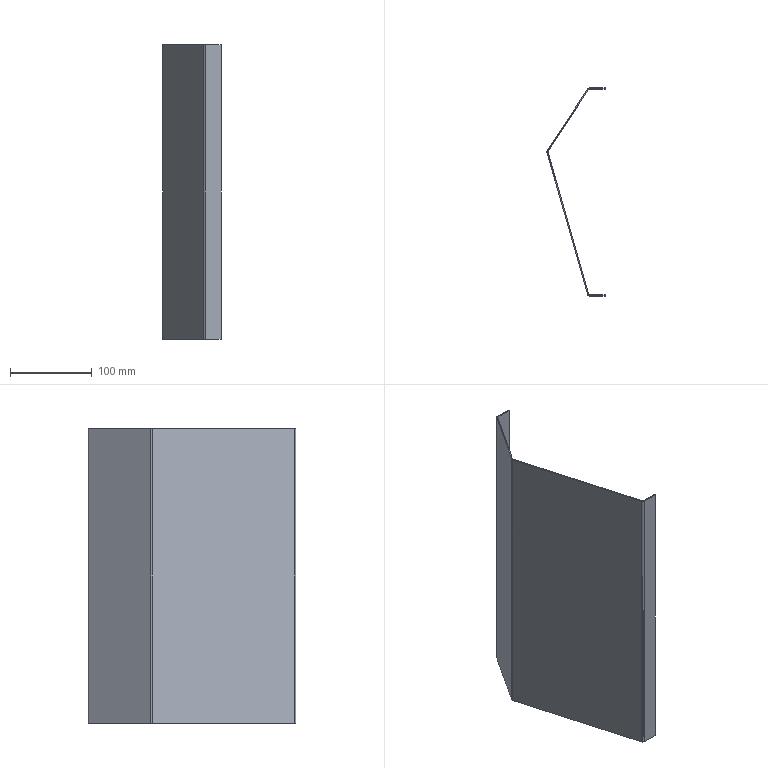Part | SolidWorks | features FlatPattern 1, SMBaseFlange 1, SheetMetal 1 | 1 solid | 30 faces | box 71.113 x 253.6 x 360 mm | volume 135935 mm3 | plane 24 | cylinder 6 | commonest cylinder face diameters 2 x3 4.4 x3
STEP:
#1=CARTESIAN_POINT('',(-12.096,249.549,30.));
#2=VERTEX_POINT('',#1);
#3=CARTESIAN_POINT('',(-13.099,250.207,30.));
#4=VERTEX_POINT('',#3);
#5=CARTESIAN_POINT('',(-12.096,249.549,30.));
#6=DIRECTION('',(-0.8361,0.5486,0.));
#7=VECTOR('',#6,1000.);
#8=LINE('',#5,#7);
#9=EDGE_CURVE('',#2,#4,#8,.T.);
#10=ORIENTED_EDGE('',*,*,#9,.F.);
#11=CARTESIAN_POINT('',(-11.26,250.,30.));
#12=VERTEX_POINT('',#11);
#13=CARTESIAN_POINT('',(-11.26,249.,30.));
#14=DIRECTION('',(0.,0.,1.));
#15=DIRECTION('',(-1.,0.,0.));
#16=AXIS2_PLACEMENT_3D('',#13,#14,#15);
#17=CIRCLE('',#16,1.);
#18=EDGE_CURVE('',#12,#2,#17,.T.);
#19=ORIENTED_EDGE('',*,*,#18,.F.);
#20=CARTESIAN_POINT('',(-11.26,251.2,30.));
#21=VERTEX_POINT('',#20);
#22=CARTESIAN_POINT('',(-11.26,251.2,30.));
#23=DIRECTION('',(0.,-1.,0.));
#24=VECTOR('',#23,1000.);
#25=LINE('',#22,#24);
#26=EDGE_CURVE('',#21,#12,#25,.T.);
#27=ORIENTED_EDGE('',*,*,#26,.F.);
#28=CARTESIAN_POINT('',(-11.26,249.,30.));
#29=DIRECTION('',(0.,0.,1.));
#30=DIRECTION('',(1.,0.,0.));
#31=AXIS2_PLACEMENT_3D('',#28,#29,#30);
#32=CIRCLE('',#31,2.2);
#33=EDGE_CURVE('',#21,#4,#32,.T.);
#34=ORIENTED_EDGE('',*,*,#33,.T.);
#35=EDGE_LOOP('',(#10,#19,#27,#34));
#36=FACE_OUTER_BOUND('',#35,.T.);
#37=CARTESIAN_POINT('',(-12.096,249.549,30.));
#38=DIRECTION('',(0.,0.,1.));
#39=DIRECTION('',(1.,0.,0.));
#40=AXIS2_PLACEMENT_3D('',#37,#38,#39);
#41=PLANE('',#40);
#42=ADVANCED_FACE('',(#36),#41,.T.);
#43=CARTESIAN_POINT('',(-61.549,174.183,30.));
#44=VERTEX_POINT('',#43);
#45=CARTESIAN_POINT('',(-11.8,250.,30.));
#46=DIRECTION('',(-0.5486,-0.8361,0.));
#47=VECTOR('',#46,1000.);
#48=LINE('',#45,#47);
#49=EDGE_CURVE('',#2,#44,#48,.T.);
#50=ORIENTED_EDGE('',*,*,#49,.F.);
#51=ORIENTED_EDGE('',*,*,#9,.T.);
#52=CARTESIAN_POINT('',(-62.552,174.841,30.));
#53=VERTEX_POINT('',#52);
#54=CARTESIAN_POINT('',(-12.803,250.658,30.));
#55=DIRECTION('',(-0.5486,-0.8361,0.));
#56=VECTOR('',#55,1000.);
#57=LINE('',#54,#56);
#58=EDGE_CURVE('',#4,#53,#57,.T.);
#59=ORIENTED_EDGE('',*,*,#58,.T.);
#60=CARTESIAN_POINT('',(-62.552,174.841,30.));
#61=DIRECTION('',(0.8361,-0.5486,0.));
#62=VECTOR('',#61,1000.);
#63=LINE('',#60,#62);
#64=EDGE_CURVE('',#53,#44,#63,.T.);
#65=ORIENTED_EDGE('',*,*,#64,.T.);
#66=EDGE_LOOP('',(#50,#51,#59,#65));
#67=FACE_OUTER_BOUND('',#66,.T.);
#68=CARTESIAN_POINT('',(-11.26,251.2,30.));
#69=DIRECTION('',(0.,0.,1.));
#70=DIRECTION('',(1.,0.,0.));
#71=AXIS2_PLACEMENT_3D('',#68,#69,#70);
#72=PLANE('',#71);
#73=ADVANCED_FACE('',(#67),#72,.T.);
#74=CARTESIAN_POINT('',(-61.674,173.36,30.));
#75=VERTEX_POINT('',#74);
#76=CARTESIAN_POINT('',(-62.828,173.03,30.));
#77=VERTEX_POINT('',#76);
#78=CARTESIAN_POINT('',(-61.674,173.36,30.));
#79=DIRECTION('',(-0.9615,-0.2747,0.));
#80=VECTOR('',#79,1000.);
#81=LINE('',#78,#80);
#82=EDGE_CURVE('',#75,#77,#81,.T.);
#83=ORIENTED_EDGE('',*,*,#82,.F.);
#84=CARTESIAN_POINT('',(-60.713,173.634,30.));
#85=DIRECTION('',(0.,0.,1.));
#86=DIRECTION('',(-1.,0.,0.));
#87=AXIS2_PLACEMENT_3D('',#84,#85,#86);
#88=CIRCLE('',#87,1.);
#89=EDGE_CURVE('',#44,#75,#88,.T.);
#90=ORIENTED_EDGE('',*,*,#89,.F.);
#91=ORIENTED_EDGE('',*,*,#64,.F.);
#92=CARTESIAN_POINT('',(-60.713,173.634,30.));
#93=DIRECTION('',(0.,0.,1.));
#94=DIRECTION('',(1.,0.,0.));
#95=AXIS2_PLACEMENT_3D('',#92,#93,#94);
#96=CIRCLE('',#95,2.2);
#97=EDGE_CURVE('',#53,#77,#96,.T.);
#98=ORIENTED_EDGE('',*,*,#97,.T.);
#99=EDGE_LOOP('',(#83,#90,#91,#98));
#100=FACE_OUTER_BOUND('',#99,.T.);
#101=CARTESIAN_POINT('',(-61.674,173.36,30.));
#102=DIRECTION('',(0.,0.,1.));
#103=DIRECTION('',(1.,0.,0.));
#104=AXIS2_PLACEMENT_3D('',#101,#102,#103);
#105=PLANE('',#104);
#106=ADVANCED_FACE('',(#100),#105,.T.);
#107=CARTESIAN_POINT('',(-12.007,-0.4747,30.));
#108=VERTEX_POINT('',#107);
#109=CARTESIAN_POINT('',(-61.8,173.8,30.));
#110=DIRECTION('',(0.2747,-0.9615,0.));
#111=VECTOR('',#110,1000.);
#112=LINE('',#109,#111);
#113=EDGE_CURVE('',#75,#108,#112,.T.);
#114=ORIENTED_EDGE('',*,*,#113,.F.);
#115=ORIENTED_EDGE('',*,*,#82,.T.);
#116=CARTESIAN_POINT('',(-13.161,-0.8044,30.));
#117=VERTEX_POINT('',#116);
#118=CARTESIAN_POINT('',(-62.954,173.47,30.));
#119=DIRECTION('',(0.2747,-0.9615,0.));
#120=VECTOR('',#119,1000.);
#121=LINE('',#118,#120);
#122=EDGE_CURVE('',#77,#117,#121,.T.);
#123=ORIENTED_EDGE('',*,*,#122,.T.);
#124=CARTESIAN_POINT('',(-13.161,-0.8044,30.));
#125=DIRECTION('',(0.9615,0.2747,0.));
#126=VECTOR('',#125,1000.);
#127=LINE('',#124,#126);
#128=EDGE_CURVE('',#117,#108,#127,.T.);
#129=ORIENTED_EDGE('',*,*,#128,.T.);
#130=EDGE_LOOP('',(#114,#115,#123,#129));
#131=FACE_OUTER_BOUND('',#130,.T.);
#132=CARTESIAN_POINT('',(-62.552,174.841,30.));
#133=DIRECTION('',(0.,0.,1.));
#134=DIRECTION('',(1.,0.,0.));
#135=AXIS2_PLACEMENT_3D('',#132,#133,#134);
#136=PLANE('',#135);
#137=ADVANCED_FACE('',(#131),#136,.T.);
#138=CARTESIAN_POINT('',(-11.046,-1.2,30.));
#139=VERTEX_POINT('',#138);
#140=CARTESIAN_POINT('',(-11.046,-2.4,30.));
#141=VERTEX_POINT('',#140);
#142=CARTESIAN_POINT('',(-11.046,-1.2,30.));
#143=DIRECTION('',(0.,-1.,0.));
#144=VECTOR('',#143,1000.);
#145=LINE('',#142,#144);
#146=EDGE_CURVE('',#139,#141,#145,.T.);
#147=ORIENTED_EDGE('',*,*,#146,.F.);
#148=CARTESIAN_POINT('',(-11.046,-0.2,30.));
#149=DIRECTION('',(0.,0.,1.));
#150=DIRECTION('',(-1.,0.,0.));
#151=AXIS2_PLACEMENT_3D('',#148,#149,#150);
#152=CIRCLE('',#151,1.);
#153=EDGE_CURVE('',#108,#139,#152,.T.);
#154=ORIENTED_EDGE('',*,*,#153,.F.);
#155=ORIENTED_EDGE('',*,*,#128,.F.);
#156=CARTESIAN_POINT('',(-11.046,-0.2,30.));
#157=DIRECTION('',(0.,0.,1.));
#158=DIRECTION('',(1.,0.,0.));
#159=AXIS2_PLACEMENT_3D('',#156,#157,#158);
#160=CIRCLE('',#159,2.2);
#161=EDGE_CURVE('',#117,#141,#160,.T.);
#162=ORIENTED_EDGE('',*,*,#161,.T.);
#163=EDGE_LOOP('',(#147,#154,#155,#162));
#164=FACE_OUTER_BOUND('',#163,.T.);
#165=CARTESIAN_POINT('',(-11.046,-1.2,30.));
#166=DIRECTION('',(0.,0.,1.));
#167=DIRECTION('',(1.,0.,0.));
#168=AXIS2_PLACEMENT_3D('',#165,#166,#167);
#169=PLANE('',#168);
#170=ADVANCED_FACE('',(#164),#169,.T.);
#171=CARTESIAN_POINT('',(8.2,-1.2,30.));
#172=VERTEX_POINT('',#171);
#173=CARTESIAN_POINT('',(-11.8,-1.2,30.));
#174=DIRECTION('',(1.,0.,0.));
#175=VECTOR('',#174,1000.);
#176=LINE('',#173,#175);
#177=EDGE_CURVE('',#139,#172,#176,.T.);
#178=ORIENTED_EDGE('',*,*,#177,.F.);
#179=ORIENTED_EDGE('',*,*,#146,.T.);
#180=CARTESIAN_POINT('',(8.2,-2.4,30.));
#181=VERTEX_POINT('',#180);
#182=CARTESIAN_POINT('',(-11.8,-2.4,30.));
#183=DIRECTION('',(1.,0.,0.));
#184=VECTOR('',#183,1000.);
#185=LINE('',#182,#184);
#186=EDGE_CURVE('',#141,#181,#185,.T.);
#187=ORIENTED_EDGE('',*,*,#186,.T.);
#188=CARTESIAN_POINT('',(8.2,-1.2,30.));
#189=DIRECTION('',(0.,-1.,0.));
#190=VECTOR('',#189,1000.);
#191=LINE('',#188,#190);
#192=EDGE_CURVE('',#172,#181,#191,.T.);
#193=ORIENTED_EDGE('',*,*,#192,.F.);
#194=EDGE_LOOP('',(#178,#179,#187,#193));
#195=FACE_OUTER_BOUND('',#194,.T.);
#196=CARTESIAN_POINT('',(-13.161,-0.8044,30.));
#197=DIRECTION('',(0.,0.,1.));
#198=DIRECTION('',(1.,0.,0.));
#199=AXIS2_PLACEMENT_3D('',#196,#197,#198);
#200=PLANE('',#199);
#201=ADVANCED_FACE('',(#195),#200,.T.);
#202=CARTESIAN_POINT('',(-11.046,-2.4,-330.));
#203=VERTEX_POINT('',#202);
#204=CARTESIAN_POINT('',(-11.046,-2.4,-593.382));
#205=DIRECTION('',(0.,0.,1.));
#206=VECTOR('',#205,1000.);
#207=LINE('',#204,#206);
#208=EDGE_CURVE('',#203,#141,#207,.T.);
#209=ORIENTED_EDGE('',*,*,#208,.F.);
#210=CARTESIAN_POINT('',(8.2,-2.4,-330.));
#211=VERTEX_POINT('',#210);
#212=CARTESIAN_POINT('',(-11.8,-2.4,-330.));
#213=DIRECTION('',(-1.,0.,0.));
#214=VECTOR('',#213,1000.);
#215=LINE('',#212,#214);
#216=EDGE_CURVE('',#211,#203,#215,.T.);
#217=ORIENTED_EDGE('',*,*,#216,.F.);
#218=CARTESIAN_POINT('',(8.2,-2.4,-593.382));
#219=DIRECTION('',(0.,0.,1.));
#220=VECTOR('',#219,1000.);
#221=LINE('',#218,#220);
#222=EDGE_CURVE('',#211,#181,#221,.T.);
#223=ORIENTED_EDGE('',*,*,#222,.T.);
#224=ORIENTED_EDGE('',*,*,#186,.F.);
#225=EDGE_LOOP('',(#209,#217,#223,#224));
#226=FACE_OUTER_BOUND('',#225,.T.);
#227=CARTESIAN_POINT('',(-11.8,-2.4,-593.382));
#228=DIRECTION('',(0.,-1.,0.));
#229=DIRECTION('',(0.,0.,-1.));
#230=AXIS2_PLACEMENT_3D('',#227,#228,#229);
#231=PLANE('',#230);
#232=ADVANCED_FACE('',(#226),#231,.T.);
#233=CARTESIAN_POINT('',(-13.161,-0.8044,-330.));
#234=VERTEX_POINT('',#233);
#235=CARTESIAN_POINT('',(-13.161,-0.8044,-593.382));
#236=DIRECTION('',(0.,0.,1.));
#237=VECTOR('',#236,1000.);
#238=LINE('',#235,#237);
#239=EDGE_CURVE('',#234,#117,#238,.T.);
#240=ORIENTED_EDGE('',*,*,#239,.F.);
#241=CARTESIAN_POINT('',(-11.046,-0.2,-330.));
#242=DIRECTION('',(0.,0.,-1.));
#243=DIRECTION('',(1.,0.,0.));
#244=AXIS2_PLACEMENT_3D('',#241,#242,#243);
#245=CIRCLE('',#244,2.2);
#246=EDGE_CURVE('',#203,#234,#245,.T.);
#247=ORIENTED_EDGE('',*,*,#246,.F.);
#248=ORIENTED_EDGE('',*,*,#208,.T.);
#249=ORIENTED_EDGE('',*,*,#161,.F.);
#250=EDGE_LOOP('',(#240,#247,#248,#249));
#251=FACE_OUTER_BOUND('',#250,.T.);
#252=CARTESIAN_POINT('',(-11.046,-0.2,-593.382));
#253=DIRECTION('',(0.,0.,1.));
#254=DIRECTION('',(1.,0.,0.));
#255=AXIS2_PLACEMENT_3D('',#252,#253,#254);
#256=CYLINDRICAL_SURFACE('',#255,2.2);
#257=ADVANCED_FACE('',(#251),#256,.T.);
#258=CARTESIAN_POINT('',(-62.828,173.03,-330.));
#259=VERTEX_POINT('',#258);
#260=CARTESIAN_POINT('',(-62.828,173.03,-593.382));
#261=DIRECTION('',(0.,0.,1.));
#262=VECTOR('',#261,1000.);
#263=LINE('',#260,#262);
#264=EDGE_CURVE('',#259,#77,#263,.T.);
#265=ORIENTED_EDGE('',*,*,#264,.F.);
#266=CARTESIAN_POINT('',(-62.954,173.47,-330.));
#267=DIRECTION('',(-0.2747,0.9615,0.));
#268=VECTOR('',#267,1000.);
#269=LINE('',#266,#268);
#270=EDGE_CURVE('',#234,#259,#269,.T.);
#271=ORIENTED_EDGE('',*,*,#270,.F.);
#272=ORIENTED_EDGE('',*,*,#239,.T.);
#273=ORIENTED_EDGE('',*,*,#122,.F.);
#274=EDGE_LOOP('',(#265,#271,#272,#273));
#275=FACE_OUTER_BOUND('',#274,.T.);
#276=CARTESIAN_POINT('',(-62.954,173.47,-593.382));
#277=DIRECTION('',(-0.9615,-0.2747,0.));
#278=DIRECTION('',(0.2747,-0.9615,0.));
#279=AXIS2_PLACEMENT_3D('',#276,#277,#278);
#280=PLANE('',#279);
#281=ADVANCED_FACE('',(#275),#280,.T.);
#282=CARTESIAN_POINT('',(-62.552,174.841,-330.));
#283=VERTEX_POINT('',#282);
#284=CARTESIAN_POINT('',(-62.552,174.841,-593.382));
#285=DIRECTION('',(0.,0.,1.));
#286=VECTOR('',#285,1000.);
#287=LINE('',#284,#286);
#288=EDGE_CURVE('',#283,#53,#287,.T.);
#289=ORIENTED_EDGE('',*,*,#288,.F.);
#290=CARTESIAN_POINT('',(-60.713,173.634,-330.));
#291=DIRECTION('',(0.,0.,-1.));
#292=DIRECTION('',(1.,0.,0.));
#293=AXIS2_PLACEMENT_3D('',#290,#291,#292);
#294=CIRCLE('',#293,2.2);
#295=EDGE_CURVE('',#259,#283,#294,.T.);
#296=ORIENTED_EDGE('',*,*,#295,.F.);
#297=ORIENTED_EDGE('',*,*,#264,.T.);
#298=ORIENTED_EDGE('',*,*,#97,.F.);
#299=EDGE_LOOP('',(#289,#296,#297,#298));
#300=FACE_OUTER_BOUND('',#299,.T.);
#301=CARTESIAN_POINT('',(-60.713,173.634,-593.382));
#302=DIRECTION('',(0.,0.,1.));
#303=DIRECTION('',(1.,0.,0.));
#304=AXIS2_PLACEMENT_3D('',#301,#302,#303);
#305=CYLINDRICAL_SURFACE('',#304,2.2);
#306=ADVANCED_FACE('',(#300),#305,.T.);
#307=CARTESIAN_POINT('',(-13.099,250.207,-330.));
#308=VERTEX_POINT('',#307);
#309=CARTESIAN_POINT('',(-13.099,250.207,-593.382));
#310=DIRECTION('',(0.,0.,1.));
#311=VECTOR('',#310,1000.);
#312=LINE('',#309,#311);
#313=EDGE_CURVE('',#308,#4,#312,.T.);
#314=ORIENTED_EDGE('',*,*,#313,.F.);
#315=CARTESIAN_POINT('',(-12.803,250.658,-330.));
#316=DIRECTION('',(0.5486,0.8361,0.));
#317=VECTOR('',#316,1000.);
#318=LINE('',#315,#317);
#319=EDGE_CURVE('',#283,#308,#318,.T.);
#320=ORIENTED_EDGE('',*,*,#319,.F.);
#321=ORIENTED_EDGE('',*,*,#288,.T.);
#322=ORIENTED_EDGE('',*,*,#58,.F.);
#323=EDGE_LOOP('',(#314,#320,#321,#322));
#324=FACE_OUTER_BOUND('',#323,.T.);
#325=CARTESIAN_POINT('',(-12.803,250.658,-593.382));
#326=DIRECTION('',(-0.8361,0.5486,0.));
#327=DIRECTION('',(-0.5486,-0.8361,0.));
#328=AXIS2_PLACEMENT_3D('',#325,#326,#327);
#329=PLANE('',#328);
#330=ADVANCED_FACE('',(#324),#329,.T.);
#331=CARTESIAN_POINT('',(-11.26,251.2,-330.));
#332=VERTEX_POINT('',#331);
#333=CARTESIAN_POINT('',(-11.26,251.2,-593.382));
#334=DIRECTION('',(0.,0.,1.));
#335=VECTOR('',#334,1000.);
#336=LINE('',#333,#335);
#337=EDGE_CURVE('',#332,#21,#336,.T.);
#338=ORIENTED_EDGE('',*,*,#337,.F.);
#339=CARTESIAN_POINT('',(-11.26,249.,-330.));
#340=DIRECTION('',(0.,0.,-1.));
#341=DIRECTION('',(1.,0.,0.));
#342=AXIS2_PLACEMENT_3D('',#339,#340,#341);
#343=CIRCLE('',#342,2.2);
#344=EDGE_CURVE('',#308,#332,#343,.T.);
#345=ORIENTED_EDGE('',*,*,#344,.F.);
#346=ORIENTED_EDGE('',*,*,#313,.T.);
#347=ORIENTED_EDGE('',*,*,#33,.F.);
#348=EDGE_LOOP('',(#338,#345,#346,#347));
#349=FACE_OUTER_BOUND('',#348,.T.);
#350=CARTESIAN_POINT('',(-11.26,249.,-593.382));
#351=DIRECTION('',(0.,0.,1.));
#352=DIRECTION('',(1.,0.,0.));
#353=AXIS2_PLACEMENT_3D('',#350,#351,#352);
#354=CYLINDRICAL_SURFACE('',#353,2.2);
#355=ADVANCED_FACE('',(#349),#354,.T.);
#356=CARTESIAN_POINT('',(8.2,251.2,-330.));
#357=VERTEX_POINT('',#356);
#358=CARTESIAN_POINT('',(8.2,251.2,30.));
#359=VERTEX_POINT('',#358);
#360=CARTESIAN_POINT('',(8.2,251.2,-593.382));
#361=DIRECTION('',(0.,0.,1.));
#362=VECTOR('',#361,1000.);
#363=LINE('',#360,#362);
#364=EDGE_CURVE('',#357,#359,#363,.T.);
#365=ORIENTED_EDGE('',*,*,#364,.F.);
#366=CARTESIAN_POINT('',(8.2,251.2,-330.));
#367=DIRECTION('',(1.,0.,0.));
#368=VECTOR('',#367,1000.);
#369=LINE('',#366,#368);
#370=EDGE_CURVE('',#332,#357,#369,.T.);
#371=ORIENTED_EDGE('',*,*,#370,.F.);
#372=ORIENTED_EDGE('',*,*,#337,.T.);
#373=CARTESIAN_POINT('',(8.2,251.2,30.));
#374=DIRECTION('',(-1.,0.,0.));
#375=VECTOR('',#374,1000.);
#376=LINE('',#373,#375);
#377=EDGE_CURVE('',#359,#21,#376,.T.);
#378=ORIENTED_EDGE('',*,*,#377,.F.);
#379=EDGE_LOOP('',(#365,#371,#372,#378));
#380=FACE_OUTER_BOUND('',#379,.T.);
#381=CARTESIAN_POINT('',(8.2,251.2,-593.382));
#382=DIRECTION('',(0.,1.,0.));
#383=DIRECTION('',(0.,0.,1.));
#384=AXIS2_PLACEMENT_3D('',#381,#382,#383);
#385=PLANE('',#384);
#386=ADVANCED_FACE('',(#380),#385,.T.);
#387=CARTESIAN_POINT('',(8.2,250.,-330.));
#388=VERTEX_POINT('',#387);
#389=CARTESIAN_POINT('',(8.2,250.,-330.));
#390=DIRECTION('',(0.,1.,0.));
#391=VECTOR('',#390,1000.);
#392=LINE('',#389,#391);
#393=EDGE_CURVE('',#388,#357,#392,.T.);
#394=ORIENTED_EDGE('',*,*,#393,.T.);
#395=ORIENTED_EDGE('',*,*,#364,.T.);
#396=CARTESIAN_POINT('',(8.2,250.,30.));
#397=VERTEX_POINT('',#396);
#398=CARTESIAN_POINT('',(8.2,251.2,30.));
#399=DIRECTION('',(0.,-1.,0.));
#400=VECTOR('',#399,1000.);
#401=LINE('',#398,#400);
#402=EDGE_CURVE('',#359,#397,#401,.T.);
#403=ORIENTED_EDGE('',*,*,#402,.T.);
#404=CARTESIAN_POINT('',(8.2,250.,-593.382));
#405=DIRECTION('',(0.,0.,1.));
#406=VECTOR('',#405,1000.);
#407=LINE('',#404,#406);
#408=EDGE_CURVE('',#388,#397,#407,.T.);
#409=ORIENTED_EDGE('',*,*,#408,.F.);
#410=EDGE_LOOP('',(#394,#395,#403,#409));
#411=FACE_OUTER_BOUND('',#410,.T.);
#412=CARTESIAN_POINT('',(8.2,251.2,-593.382));
#413=DIRECTION('',(-1.,0.,0.));
#414=DIRECTION('',(0.,0.,1.));
#415=AXIS2_PLACEMENT_3D('',#412,#413,#414);
#416=PLANE('',#415);
#417=ADVANCED_FACE('',(#411),#416,.F.);
#418=CARTESIAN_POINT('',(-11.26,250.,-330.));
#419=VERTEX_POINT('',#418);
#420=CARTESIAN_POINT('',(8.2,250.,-330.));
#421=DIRECTION('',(1.,0.,0.));
#422=VECTOR('',#421,1000.);
#423=LINE('',#420,#422);
#424=EDGE_CURVE('',#419,#388,#423,.T.);
#425=ORIENTED_EDGE('',*,*,#424,.T.);
#426=ORIENTED_EDGE('',*,*,#408,.T.);
#427=CARTESIAN_POINT('',(8.2,250.,30.));
#428=DIRECTION('',(-1.,0.,0.));
#429=VECTOR('',#428,1000.);
#430=LINE('',#427,#429);
#431=EDGE_CURVE('',#397,#12,#430,.T.);
#432=ORIENTED_EDGE('',*,*,#431,.T.);
#433=CARTESIAN_POINT('',(-11.26,250.,-593.382));
#434=DIRECTION('',(0.,0.,1.));
#435=VECTOR('',#434,1000.);
#436=LINE('',#433,#435);
#437=EDGE_CURVE('',#419,#12,#436,.T.);
#438=ORIENTED_EDGE('',*,*,#437,.F.);
#439=EDGE_LOOP('',(#425,#426,#432,#438));
#440=FACE_OUTER_BOUND('',#439,.T.);
#441=CARTESIAN_POINT('',(8.2,250.,-593.382));
#442=DIRECTION('',(0.,1.,0.));
#443=DIRECTION('',(0.,0.,1.));
#444=AXIS2_PLACEMENT_3D('',#441,#442,#443);
#445=PLANE('',#444);
#446=ADVANCED_FACE('',(#440),#445,.F.);
#447=CARTESIAN_POINT('',(-12.096,249.549,-330.));
#448=VERTEX_POINT('',#447);
#449=CARTESIAN_POINT('',(-11.26,249.,-330.));
#450=DIRECTION('',(0.,0.,-1.));
#451=DIRECTION('',(1.,0.,0.));
#452=AXIS2_PLACEMENT_3D('',#449,#450,#451);
#453=CIRCLE('',#452,1.);
#454=EDGE_CURVE('',#448,#419,#453,.T.);
#455=ORIENTED_EDGE('',*,*,#454,.T.);
#456=ORIENTED_EDGE('',*,*,#437,.T.);
#457=ORIENTED_EDGE('',*,*,#18,.T.);
#458=CARTESIAN_POINT('',(-12.096,249.549,-593.382));
#459=DIRECTION('',(0.,0.,1.));
#460=VECTOR('',#459,1000.);
#461=LINE('',#458,#460);
#462=EDGE_CURVE('',#448,#2,#461,.T.);
#463=ORIENTED_EDGE('',*,*,#462,.F.);
#464=EDGE_LOOP('',(#455,#456,#457,#463));
#465=FACE_OUTER_BOUND('',#464,.T.);
#466=CARTESIAN_POINT('',(-11.26,249.,-593.382));
#467=DIRECTION('',(0.,0.,1.));
#468=DIRECTION('',(1.,0.,0.));
#469=AXIS2_PLACEMENT_3D('',#466,#467,#468);
#470=CYLINDRICAL_SURFACE('',#469,1.);
#471=ADVANCED_FACE('',(#465),#470,.F.);
#472=CARTESIAN_POINT('',(-61.549,174.183,-330.));
#473=VERTEX_POINT('',#472);
#474=CARTESIAN_POINT('',(-11.8,250.,-330.));
#475=DIRECTION('',(0.5486,0.8361,0.));
#476=VECTOR('',#475,1000.);
#477=LINE('',#474,#476);
#478=EDGE_CURVE('',#473,#448,#477,.T.);
#479=ORIENTED_EDGE('',*,*,#478,.T.);
#480=ORIENTED_EDGE('',*,*,#462,.T.);
#481=ORIENTED_EDGE('',*,*,#49,.T.);
#482=CARTESIAN_POINT('',(-61.549,174.183,-593.382));
#483=DIRECTION('',(0.,0.,1.));
#484=VECTOR('',#483,1000.);
#485=LINE('',#482,#484);
#486=EDGE_CURVE('',#473,#44,#485,.T.);
#487=ORIENTED_EDGE('',*,*,#486,.F.);
#488=EDGE_LOOP('',(#479,#480,#481,#487));
#489=FACE_OUTER_BOUND('',#488,.T.);
#490=CARTESIAN_POINT('',(-11.8,250.,-593.382));
#491=DIRECTION('',(-0.8361,0.5486,0.));
#492=DIRECTION('',(-0.5486,-0.8361,0.));
#493=AXIS2_PLACEMENT_3D('',#490,#491,#492);
#494=PLANE('',#493);
#495=ADVANCED_FACE('',(#489),#494,.F.);
#496=CARTESIAN_POINT('',(-61.674,173.36,-330.));
#497=VERTEX_POINT('',#496);
#498=CARTESIAN_POINT('',(-60.713,173.634,-330.));
#499=DIRECTION('',(0.,0.,-1.));
#500=DIRECTION('',(1.,0.,0.));
#501=AXIS2_PLACEMENT_3D('',#498,#499,#500);
#502=CIRCLE('',#501,1.);
#503=EDGE_CURVE('',#497,#473,#502,.T.);
#504=ORIENTED_EDGE('',*,*,#503,.T.);
#505=ORIENTED_EDGE('',*,*,#486,.T.);
#506=ORIENTED_EDGE('',*,*,#89,.T.);
#507=CARTESIAN_POINT('',(-61.674,173.36,-593.382));
#508=DIRECTION('',(0.,0.,1.));
#509=VECTOR('',#508,1000.);
#510=LINE('',#507,#509);
#511=EDGE_CURVE('',#497,#75,#510,.T.);
#512=ORIENTED_EDGE('',*,*,#511,.F.);
#513=EDGE_LOOP('',(#504,#505,#506,#512));
#514=FACE_OUTER_BOUND('',#513,.T.);
#515=CARTESIAN_POINT('',(-60.713,173.634,-593.382));
#516=DIRECTION('',(0.,0.,1.));
#517=DIRECTION('',(1.,0.,0.));
#518=AXIS2_PLACEMENT_3D('',#515,#516,#517);
#519=CYLINDRICAL_SURFACE('',#518,1.);
#520=ADVANCED_FACE('',(#514),#519,.F.);
#521=CARTESIAN_POINT('',(-12.007,-0.4747,-330.));
#522=VERTEX_POINT('',#521);
#523=CARTESIAN_POINT('',(-61.8,173.8,-330.));
#524=DIRECTION('',(-0.2747,0.9615,0.));
#525=VECTOR('',#524,1000.);
#526=LINE('',#523,#525);
#527=EDGE_CURVE('',#522,#497,#526,.T.);
#528=ORIENTED_EDGE('',*,*,#527,.T.);
#529=ORIENTED_EDGE('',*,*,#511,.T.);
#530=ORIENTED_EDGE('',*,*,#113,.T.);
#531=CARTESIAN_POINT('',(-12.007,-0.4747,-593.382));
#532=DIRECTION('',(0.,0.,1.));
#533=VECTOR('',#532,1000.);
#534=LINE('',#531,#533);
#535=EDGE_CURVE('',#522,#108,#534,.T.);
#536=ORIENTED_EDGE('',*,*,#535,.F.);
#537=EDGE_LOOP('',(#528,#529,#530,#536));
#538=FACE_OUTER_BOUND('',#537,.T.);
#539=CARTESIAN_POINT('',(-61.8,173.8,-593.382));
#540=DIRECTION('',(-0.9615,-0.2747,0.));
#541=DIRECTION('',(0.2747,-0.9615,0.));
#542=AXIS2_PLACEMENT_3D('',#539,#540,#541);
#543=PLANE('',#542);
#544=ADVANCED_FACE('',(#538),#543,.F.);
#545=CARTESIAN_POINT('',(-11.046,-1.2,-330.));
#546=VERTEX_POINT('',#545);
#547=CARTESIAN_POINT('',(-11.046,-0.2,-330.));
#548=DIRECTION('',(0.,0.,-1.));
#549=DIRECTION('',(1.,0.,0.));
#550=AXIS2_PLACEMENT_3D('',#547,#548,#549);
#551=CIRCLE('',#550,1.);
#552=EDGE_CURVE('',#546,#522,#551,.T.);
#553=ORIENTED_EDGE('',*,*,#552,.T.);
#554=ORIENTED_EDGE('',*,*,#535,.T.);
#555=ORIENTED_EDGE('',*,*,#153,.T.);
#556=CARTESIAN_POINT('',(-11.046,-1.2,-593.382));
#557=DIRECTION('',(0.,0.,1.));
#558=VECTOR('',#557,1000.);
#559=LINE('',#556,#558);
#560=EDGE_CURVE('',#546,#139,#559,.T.);
#561=ORIENTED_EDGE('',*,*,#560,.F.);
#562=EDGE_LOOP('',(#553,#554,#555,#561));
#563=FACE_OUTER_BOUND('',#562,.T.);
#564=CARTESIAN_POINT('',(-11.046,-0.2,-593.382));
#565=DIRECTION('',(0.,0.,1.));
#566=DIRECTION('',(1.,0.,0.));
#567=AXIS2_PLACEMENT_3D('',#564,#565,#566);
#568=CYLINDRICAL_SURFACE('',#567,1.);
#569=ADVANCED_FACE('',(#563),#568,.F.);
#570=CARTESIAN_POINT('',(8.2,-1.2,-330.));
#571=VERTEX_POINT('',#570);
#572=CARTESIAN_POINT('',(-11.8,-1.2,-330.));
#573=DIRECTION('',(-1.,0.,0.));
#574=VECTOR('',#573,1000.);
#575=LINE('',#572,#574);
#576=EDGE_CURVE('',#571,#546,#575,.T.);
#577=ORIENTED_EDGE('',*,*,#576,.T.);
#578=ORIENTED_EDGE('',*,*,#560,.T.);
#579=ORIENTED_EDGE('',*,*,#177,.T.);
#580=CARTESIAN_POINT('',(8.2,-1.2,-593.382));
#581=DIRECTION('',(0.,0.,1.));
#582=VECTOR('',#581,1000.);
#583=LINE('',#580,#582);
#584=EDGE_CURVE('',#571,#172,#583,.T.);
#585=ORIENTED_EDGE('',*,*,#584,.F.);
#586=EDGE_LOOP('',(#577,#578,#579,#585));
#587=FACE_OUTER_BOUND('',#586,.T.);
#588=CARTESIAN_POINT('',(-11.8,-1.2,-593.382));
#589=DIRECTION('',(0.,-1.,0.));
#590=DIRECTION('',(0.,0.,-1.));
#591=AXIS2_PLACEMENT_3D('',#588,#589,#590);
#592=PLANE('',#591);
#593=ADVANCED_FACE('',(#587),#592,.F.);
#594=CARTESIAN_POINT('',(8.2,-2.4,-330.));
#595=DIRECTION('',(0.,1.,0.));
#596=VECTOR('',#595,1000.);
#597=LINE('',#594,#596);
#598=EDGE_CURVE('',#211,#571,#597,.T.);
#599=ORIENTED_EDGE('',*,*,#598,.T.);
#600=ORIENTED_EDGE('',*,*,#584,.T.);
#601=ORIENTED_EDGE('',*,*,#192,.T.);
#602=ORIENTED_EDGE('',*,*,#222,.F.);
#603=EDGE_LOOP('',(#599,#600,#601,#602));
#604=FACE_OUTER_BOUND('',#603,.T.);
#605=CARTESIAN_POINT('',(8.2,-1.2,-593.382));
#606=DIRECTION('',(-1.,0.,0.));
#607=DIRECTION('',(0.,0.,1.));
#608=AXIS2_PLACEMENT_3D('',#605,#606,#607);
#609=PLANE('',#608);
#610=ADVANCED_FACE('',(#604),#609,.F.);
#611=ORIENTED_EDGE('',*,*,#377,.T.);
#612=ORIENTED_EDGE('',*,*,#26,.T.);
#613=ORIENTED_EDGE('',*,*,#431,.F.);
#614=ORIENTED_EDGE('',*,*,#402,.F.);
#615=EDGE_LOOP('',(#611,#612,#613,#614));
#616=FACE_OUTER_BOUND('',#615,.T.);
#617=CARTESIAN_POINT('',(-11.046,-0.2,30.));
#618=DIRECTION('',(0.,0.,-1.));
#619=DIRECTION('',(-1.,0.,0.));
#620=AXIS2_PLACEMENT_3D('',#617,#618,#619);
#621=PLANE('',#620);
#622=ADVANCED_FACE('',(#616),#621,.F.);
#623=ORIENTED_EDGE('',*,*,#216,.T.);
#624=CARTESIAN_POINT('',(-11.046,-2.4,-330.));
#625=DIRECTION('',(0.,1.,0.));
#626=VECTOR('',#625,1000.);
#627=LINE('',#624,#626);
#628=EDGE_CURVE('',#203,#546,#627,.T.);
#629=ORIENTED_EDGE('',*,*,#628,.T.);
#630=ORIENTED_EDGE('',*,*,#576,.F.);
#631=ORIENTED_EDGE('',*,*,#598,.F.);
#632=EDGE_LOOP('',(#623,#629,#630,#631));
#633=FACE_OUTER_BOUND('',#632,.T.);
#634=CARTESIAN_POINT('',(-11.8,-2.4,-330.));
#635=DIRECTION('',(0.,0.,1.));
#636=DIRECTION('',(-1.,0.,0.));
#637=AXIS2_PLACEMENT_3D('',#634,#635,#636);
#638=PLANE('',#637);
#639=ADVANCED_FACE('',(#633),#638,.F.);
#640=CARTESIAN_POINT('',(-61.674,173.36,-330.));
#641=DIRECTION('',(-0.9615,-0.2747,0.));
#642=VECTOR('',#641,1000.);
#643=LINE('',#640,#642);
#644=EDGE_CURVE('',#497,#259,#643,.T.);
#645=ORIENTED_EDGE('',*,*,#644,.F.);
#646=ORIENTED_EDGE('',*,*,#527,.F.);
#647=CARTESIAN_POINT('',(-12.007,-0.4747,-330.));
#648=DIRECTION('',(-0.9615,-0.2747,0.));
#649=VECTOR('',#648,1000.);
#650=LINE('',#647,#649);
#651=EDGE_CURVE('',#522,#234,#650,.T.);
#652=ORIENTED_EDGE('',*,*,#651,.T.);
#653=ORIENTED_EDGE('',*,*,#270,.T.);
#654=EDGE_LOOP('',(#645,#646,#652,#653));
#655=FACE_OUTER_BOUND('',#654,.T.);
#656=CARTESIAN_POINT('',(-61.8,173.8,-330.));
#657=DIRECTION('',(0.,0.,1.));
#658=DIRECTION('',(-0.2747,0.9615,0.));
#659=AXIS2_PLACEMENT_3D('',#656,#657,#658);
#660=PLANE('',#659);
#661=ADVANCED_FACE('',(#655),#660,.F.);
#662=CARTESIAN_POINT('',(-12.096,249.549,-330.));
#663=DIRECTION('',(-0.8361,0.5486,0.));
#664=VECTOR('',#663,1000.);
#665=LINE('',#662,#664);
#666=EDGE_CURVE('',#448,#308,#665,.T.);
#667=ORIENTED_EDGE('',*,*,#666,.F.);
#668=ORIENTED_EDGE('',*,*,#478,.F.);
#669=CARTESIAN_POINT('',(-61.549,174.183,-330.));
#670=DIRECTION('',(-0.8361,0.5486,0.));
#671=VECTOR('',#670,1000.);
#672=LINE('',#669,#671);
#673=EDGE_CURVE('',#473,#283,#672,.T.);
#674=ORIENTED_EDGE('',*,*,#673,.T.);
#675=ORIENTED_EDGE('',*,*,#319,.T.);
#676=EDGE_LOOP('',(#667,#668,#674,#675));
#677=FACE_OUTER_BOUND('',#676,.T.);
#678=CARTESIAN_POINT('',(-11.8,250.,-330.));
#679=DIRECTION('',(0.,0.,1.));
#680=DIRECTION('',(0.5486,0.8361,0.));
#681=AXIS2_PLACEMENT_3D('',#678,#679,#680);
#682=PLANE('',#681);
#683=ADVANCED_FACE('',(#677),#682,.F.);
#684=ORIENTED_EDGE('',*,*,#393,.F.);
#685=ORIENTED_EDGE('',*,*,#424,.F.);
#686=CARTESIAN_POINT('',(-11.26,250.,-330.));
#687=DIRECTION('',(0.,1.,0.));
#688=VECTOR('',#687,1000.);
#689=LINE('',#686,#688);
#690=EDGE_CURVE('',#419,#332,#689,.T.);
#691=ORIENTED_EDGE('',*,*,#690,.T.);
#692=ORIENTED_EDGE('',*,*,#370,.T.);
#693=EDGE_LOOP('',(#684,#685,#691,#692));
#694=FACE_OUTER_BOUND('',#693,.T.);
#695=CARTESIAN_POINT('',(8.2,250.,-330.));
#696=DIRECTION('',(0.,0.,1.));
#697=DIRECTION('',(1.,0.,0.));
#698=AXIS2_PLACEMENT_3D('',#695,#696,#697);
#699=PLANE('',#698);
#700=ADVANCED_FACE('',(#694),#699,.F.);
#701=ORIENTED_EDGE('',*,*,#690,.F.);
#702=ORIENTED_EDGE('',*,*,#454,.F.);
#703=ORIENTED_EDGE('',*,*,#666,.T.);
#704=ORIENTED_EDGE('',*,*,#344,.T.);
#705=EDGE_LOOP('',(#701,#702,#703,#704));
#706=FACE_OUTER_BOUND('',#705,.T.);
#707=CARTESIAN_POINT('',(-11.26,249.,-330.));
#708=DIRECTION('',(0.,0.,-1.));
#709=DIRECTION('',(-1.,0.,0.));
#710=AXIS2_PLACEMENT_3D('',#707,#708,#709);
#711=PLANE('',#710);
#712=ADVANCED_FACE('',(#706),#711,.T.);
#713=ORIENTED_EDGE('',*,*,#673,.F.);
#714=ORIENTED_EDGE('',*,*,#503,.F.);
#715=ORIENTED_EDGE('',*,*,#644,.T.);
#716=ORIENTED_EDGE('',*,*,#295,.T.);
#717=EDGE_LOOP('',(#713,#714,#715,#716));
#718=FACE_OUTER_BOUND('',#717,.T.);
#719=CARTESIAN_POINT('',(-60.713,173.634,-330.));
#720=DIRECTION('',(0.,0.,-1.));
#721=DIRECTION('',(-1.,0.,0.));
#722=AXIS2_PLACEMENT_3D('',#719,#720,#721);
#723=PLANE('',#722);
#724=ADVANCED_FACE('',(#718),#723,.T.);
#725=ORIENTED_EDGE('',*,*,#651,.F.);
#726=ORIENTED_EDGE('',*,*,#552,.F.);
#727=ORIENTED_EDGE('',*,*,#628,.F.);
#728=ORIENTED_EDGE('',*,*,#246,.T.);
#729=EDGE_LOOP('',(#725,#726,#727,#728));
#730=FACE_OUTER_BOUND('',#729,.T.);
#731=CARTESIAN_POINT('',(-11.046,-0.2,-330.));
#732=DIRECTION('',(0.,0.,-1.));
#733=DIRECTION('',(-1.,0.,0.));
#734=AXIS2_PLACEMENT_3D('',#731,#732,#733);
#735=PLANE('',#734);
#736=ADVANCED_FACE('',(#730),#735,.T.);
#737=CLOSED_SHELL('',(#42,#73,#106,#137,#170,#201,#232,#257,#281,#306,#330,#355,#386,#417,#446,#471,#495,#520,#544,#569,#593,#610,#622,#639,#661,#683,#700,#712,#724,#736));
#738=MANIFOLD_SOLID_BREP('',#737);
#739=CARTESIAN_POINT('',(0.,0.,0.));
#740=DIRECTION('',(0.,0.,1.));
#741=DIRECTION('',(1.,0.,0.));
#742=AXIS2_PLACEMENT_3D('',#739,#740,#741);
#743=(LENGTH_UNIT()NAMED_UNIT(*)SI_UNIT(.MILLI.,.METRE.));
#744=UNCERTAINTY_MEASURE_WITH_UNIT(LENGTH_MEASURE(0.00001),#743,'','');
#745=(NAMED_UNIT(*)PLANE_ANGLE_UNIT()SI_UNIT($,.RADIAN.));
#746=(NAMED_UNIT(*)SI_UNIT($,.STERADIAN.)SOLID_ANGLE_UNIT());
#747=(GEOMETRIC_REPRESENTATION_CONTEXT(3)GLOBAL_UNCERTAINTY_ASSIGNED_CONTEXT((#744))GLOBAL_UNIT_ASSIGNED_CONTEXT((#743,#745,#746))REPRESENTATION_CONTEXT('',''));
#748=ADVANCED_BREP_SHAPE_REPRESENTATION('',(#738,#742),#747);